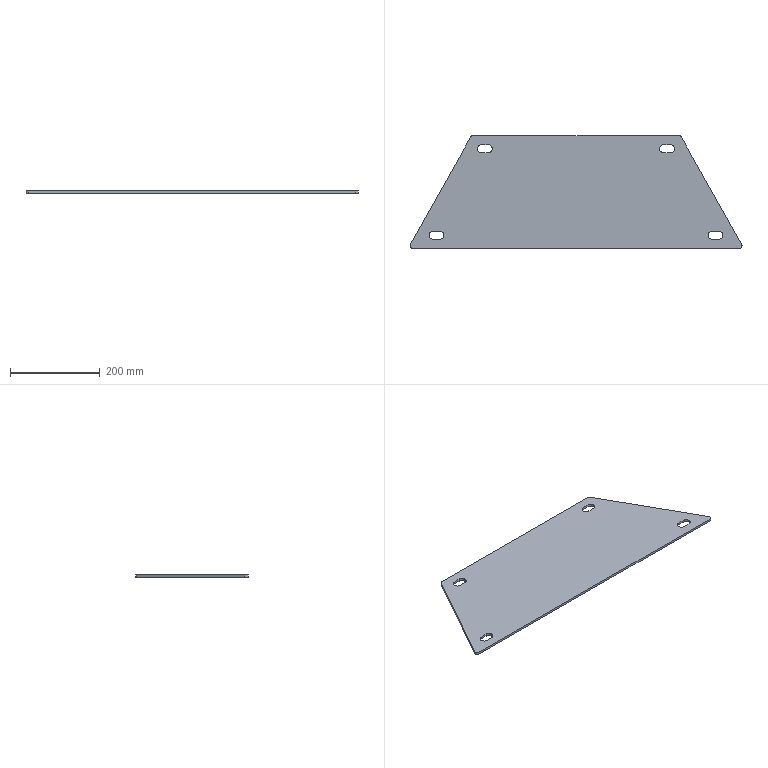Part | SolidWorks | features FlatPattern 1, SMBaseFlange 1, SheetMetal 1 | 1 solid | 31 faces | box 737.939 x 250 x 5 mm | volume 745580 mm3 | cylinder 17 | plane 14 | commonest cylinder face diameters 18 x12 10 x5
STEP:
#1=CARTESIAN_POINT('',(326.5,-96.,-5.));
#2=VERTEX_POINT('',#1);
#3=CARTESIAN_POINT('',(317.5,-87.,-5.));
#4=VERTEX_POINT('',#3);
#5=CARTESIAN_POINT('',(317.5,-96.,-5.));
#6=DIRECTION('',(0.,0.,1.));
#7=DIRECTION('',(1.,0.,0.));
#8=AXIS2_PLACEMENT_3D('',#5,#6,#7);
#9=CIRCLE('',#8,9.);
#10=EDGE_CURVE('',#2,#4,#9,.T.);
#11=ORIENTED_EDGE('',*,*,#10,.F.);
#12=CARTESIAN_POINT('',(326.5,-96.,0.));
#13=VERTEX_POINT('',#12);
#14=CARTESIAN_POINT('',(326.5,-96.,-5.));
#15=DIRECTION('',(0.,0.,1.));
#16=VECTOR('',#15,1000.);
#17=LINE('',#14,#16);
#18=EDGE_CURVE('',#2,#13,#17,.T.);
#19=ORIENTED_EDGE('',*,*,#18,.T.);
#20=CARTESIAN_POINT('',(317.5,-87.,0.));
#21=VERTEX_POINT('',#20);
#22=CARTESIAN_POINT('',(317.5,-96.,0.));
#23=DIRECTION('',(0.,0.,1.));
#24=DIRECTION('',(1.,0.,0.));
#25=AXIS2_PLACEMENT_3D('',#22,#23,#24);
#26=CIRCLE('',#25,9.);
#27=EDGE_CURVE('',#13,#21,#26,.T.);
#28=ORIENTED_EDGE('',*,*,#27,.T.);
#29=CARTESIAN_POINT('',(317.5,-87.,-5.));
#30=DIRECTION('',(0.,0.,1.));
#31=VECTOR('',#30,1000.);
#32=LINE('',#29,#31);
#33=EDGE_CURVE('',#4,#21,#32,.T.);
#34=ORIENTED_EDGE('',*,*,#33,.F.);
#35=EDGE_LOOP('',(#11,#19,#28,#34));
#36=FACE_OUTER_BOUND('',#35,.T.);
#37=CARTESIAN_POINT('',(317.5,-96.,-5.));
#38=DIRECTION('',(0.,0.,1.));
#39=DIRECTION('',(1.,0.,0.));
#40=AXIS2_PLACEMENT_3D('',#37,#38,#39);
#41=CYLINDRICAL_SURFACE('',#40,9.);
#42=ADVANCED_FACE('',(#36),#41,.F.);
#43=CARTESIAN_POINT('',(-293.5,-96.,-5.));
#44=VERTEX_POINT('',#43);
#45=CARTESIAN_POINT('',(-302.5,-87.,-5.));
#46=VERTEX_POINT('',#45);
#47=CARTESIAN_POINT('',(-302.5,-96.,-5.));
#48=DIRECTION('',(0.,0.,1.));
#49=DIRECTION('',(1.,0.,0.));
#50=AXIS2_PLACEMENT_3D('',#47,#48,#49);
#51=CIRCLE('',#50,9.);
#52=EDGE_CURVE('',#44,#46,#51,.T.);
#53=ORIENTED_EDGE('',*,*,#52,.F.);
#54=CARTESIAN_POINT('',(-293.5,-96.,0.));
#55=VERTEX_POINT('',#54);
#56=CARTESIAN_POINT('',(-293.5,-96.,-5.));
#57=DIRECTION('',(0.,0.,1.));
#58=VECTOR('',#57,1000.);
#59=LINE('',#56,#58);
#60=EDGE_CURVE('',#44,#55,#59,.T.);
#61=ORIENTED_EDGE('',*,*,#60,.T.);
#62=CARTESIAN_POINT('',(-302.5,-87.,0.));
#63=VERTEX_POINT('',#62);
#64=CARTESIAN_POINT('',(-302.5,-96.,0.));
#65=DIRECTION('',(0.,0.,1.));
#66=DIRECTION('',(1.,0.,0.));
#67=AXIS2_PLACEMENT_3D('',#64,#65,#66);
#68=CIRCLE('',#67,9.);
#69=EDGE_CURVE('',#55,#63,#68,.T.);
#70=ORIENTED_EDGE('',*,*,#69,.T.);
#71=CARTESIAN_POINT('',(-302.5,-87.,-5.));
#72=DIRECTION('',(0.,0.,1.));
#73=VECTOR('',#72,1000.);
#74=LINE('',#71,#73);
#75=EDGE_CURVE('',#46,#63,#74,.T.);
#76=ORIENTED_EDGE('',*,*,#75,.F.);
#77=EDGE_LOOP('',(#53,#61,#70,#76));
#78=FACE_OUTER_BOUND('',#77,.T.);
#79=CARTESIAN_POINT('',(-302.5,-96.,-5.));
#80=DIRECTION('',(0.,0.,1.));
#81=DIRECTION('',(1.,0.,0.));
#82=AXIS2_PLACEMENT_3D('',#79,#80,#81);
#83=CYLINDRICAL_SURFACE('',#82,9.);
#84=ADVANCED_FACE('',(#78),#83,.F.);
#85=CARTESIAN_POINT('',(219.,96.,-5.));
#86=VERTEX_POINT('',#85);
#87=CARTESIAN_POINT('',(210.,105.,-5.));
#88=VERTEX_POINT('',#87);
#89=CARTESIAN_POINT('',(210.,96.,-5.));
#90=DIRECTION('',(0.,0.,1.));
#91=DIRECTION('',(1.,0.,0.));
#92=AXIS2_PLACEMENT_3D('',#89,#90,#91);
#93=CIRCLE('',#92,9.);
#94=EDGE_CURVE('',#86,#88,#93,.T.);
#95=ORIENTED_EDGE('',*,*,#94,.F.);
#96=CARTESIAN_POINT('',(219.,96.,0.));
#97=VERTEX_POINT('',#96);
#98=CARTESIAN_POINT('',(219.,96.,-5.));
#99=DIRECTION('',(0.,0.,1.));
#100=VECTOR('',#99,1000.);
#101=LINE('',#98,#100);
#102=EDGE_CURVE('',#86,#97,#101,.T.);
#103=ORIENTED_EDGE('',*,*,#102,.T.);
#104=CARTESIAN_POINT('',(210.,105.,0.));
#105=VERTEX_POINT('',#104);
#106=CARTESIAN_POINT('',(210.,96.,0.));
#107=DIRECTION('',(0.,0.,1.));
#108=DIRECTION('',(1.,0.,0.));
#109=AXIS2_PLACEMENT_3D('',#106,#107,#108);
#110=CIRCLE('',#109,9.);
#111=EDGE_CURVE('',#97,#105,#110,.T.);
#112=ORIENTED_EDGE('',*,*,#111,.T.);
#113=CARTESIAN_POINT('',(210.,105.,-5.));
#114=DIRECTION('',(0.,0.,1.));
#115=VECTOR('',#114,1000.);
#116=LINE('',#113,#115);
#117=EDGE_CURVE('',#88,#105,#116,.T.);
#118=ORIENTED_EDGE('',*,*,#117,.F.);
#119=EDGE_LOOP('',(#95,#103,#112,#118));
#120=FACE_OUTER_BOUND('',#119,.T.);
#121=CARTESIAN_POINT('',(210.,96.,-5.));
#122=DIRECTION('',(0.,0.,1.));
#123=DIRECTION('',(1.,0.,0.));
#124=AXIS2_PLACEMENT_3D('',#121,#122,#123);
#125=CYLINDRICAL_SURFACE('',#124,9.);
#126=ADVANCED_FACE('',(#120),#125,.F.);
#127=CARTESIAN_POINT('',(-186.,96.,-5.));
#128=VERTEX_POINT('',#127);
#129=CARTESIAN_POINT('',(-195.,105.,-5.));
#130=VERTEX_POINT('',#129);
#131=CARTESIAN_POINT('',(-195.,96.,-5.));
#132=DIRECTION('',(0.,0.,1.));
#133=DIRECTION('',(1.,0.,0.));
#134=AXIS2_PLACEMENT_3D('',#131,#132,#133);
#135=CIRCLE('',#134,9.);
#136=EDGE_CURVE('',#128,#130,#135,.T.);
#137=ORIENTED_EDGE('',*,*,#136,.F.);
#138=CARTESIAN_POINT('',(-186.,96.,0.));
#139=VERTEX_POINT('',#138);
#140=CARTESIAN_POINT('',(-186.,96.,-5.));
#141=DIRECTION('',(0.,0.,1.));
#142=VECTOR('',#141,1000.);
#143=LINE('',#140,#142);
#144=EDGE_CURVE('',#128,#139,#143,.T.);
#145=ORIENTED_EDGE('',*,*,#144,.T.);
#146=CARTESIAN_POINT('',(-195.,105.,0.));
#147=VERTEX_POINT('',#146);
#148=CARTESIAN_POINT('',(-195.,96.,0.));
#149=DIRECTION('',(0.,0.,1.));
#150=DIRECTION('',(1.,0.,0.));
#151=AXIS2_PLACEMENT_3D('',#148,#149,#150);
#152=CIRCLE('',#151,9.);
#153=EDGE_CURVE('',#139,#147,#152,.T.);
#154=ORIENTED_EDGE('',*,*,#153,.T.);
#155=CARTESIAN_POINT('',(-195.,105.,-5.));
#156=DIRECTION('',(0.,0.,1.));
#157=VECTOR('',#156,1000.);
#158=LINE('',#155,#157);
#159=EDGE_CURVE('',#130,#147,#158,.T.);
#160=ORIENTED_EDGE('',*,*,#159,.F.);
#161=EDGE_LOOP('',(#137,#145,#154,#160));
#162=FACE_OUTER_BOUND('',#161,.T.);
#163=CARTESIAN_POINT('',(-195.,96.,-5.));
#164=DIRECTION('',(0.,0.,1.));
#165=DIRECTION('',(1.,0.,0.));
#166=AXIS2_PLACEMENT_3D('',#163,#164,#165);
#167=CYLINDRICAL_SURFACE('',#166,9.);
#168=ADVANCED_FACE('',(#162),#167,.F.);
#169=CARTESIAN_POINT('',(363.969,-125.,-5.));
#170=VERTEX_POINT('',#169);
#171=CARTESIAN_POINT('',(368.969,-120.,-5.));
#172=VERTEX_POINT('',#171);
#173=CARTESIAN_POINT('',(363.969,-120.,-5.));
#174=DIRECTION('',(0.,0.,1.));
#175=DIRECTION('',(-1.,0.,0.));
#176=AXIS2_PLACEMENT_3D('',#173,#174,#175);
#177=CIRCLE('',#176,5.);
#178=EDGE_CURVE('',#170,#172,#177,.T.);
#179=ORIENTED_EDGE('',*,*,#178,.T.);
#180=CARTESIAN_POINT('',(368.969,-120.,0.));
#181=VERTEX_POINT('',#180);
#182=CARTESIAN_POINT('',(368.969,-120.,-5.));
#183=DIRECTION('',(0.,0.,1.));
#184=VECTOR('',#183,1000.);
#185=LINE('',#182,#184);
#186=EDGE_CURVE('',#172,#181,#185,.T.);
#187=ORIENTED_EDGE('',*,*,#186,.T.);
#188=CARTESIAN_POINT('',(363.969,-125.,0.));
#189=VERTEX_POINT('',#188);
#190=CARTESIAN_POINT('',(363.969,-120.,0.));
#191=DIRECTION('',(0.,0.,1.));
#192=DIRECTION('',(-1.,0.,0.));
#193=AXIS2_PLACEMENT_3D('',#190,#191,#192);
#194=CIRCLE('',#193,5.);
#195=EDGE_CURVE('',#189,#181,#194,.T.);
#196=ORIENTED_EDGE('',*,*,#195,.F.);
#197=CARTESIAN_POINT('',(363.969,-125.,-5.));
#198=DIRECTION('',(0.,0.,1.));
#199=VECTOR('',#198,1000.);
#200=LINE('',#197,#199);
#201=EDGE_CURVE('',#170,#189,#200,.T.);
#202=ORIENTED_EDGE('',*,*,#201,.F.);
#203=EDGE_LOOP('',(#179,#187,#196,#202));
#204=FACE_OUTER_BOUND('',#203,.T.);
#205=CARTESIAN_POINT('',(363.969,-120.,-5.));
#206=DIRECTION('',(0.,0.,1.));
#207=DIRECTION('',(1.,0.,0.));
#208=AXIS2_PLACEMENT_3D('',#205,#206,#207);
#209=CYLINDRICAL_SURFACE('',#208,5.);
#210=ADVANCED_FACE('',(#204),#209,.T.);
#211=CARTESIAN_POINT('',(-229.569,125.,0.));
#212=VERTEX_POINT('',#211);
#213=CARTESIAN_POINT('',(-233.932,122.443,0.));
#214=VERTEX_POINT('',#213);
#215=CARTESIAN_POINT('',(-229.569,120.,0.));
#216=DIRECTION('',(0.,0.,1.));
#217=DIRECTION('',(1.,0.,0.));
#218=AXIS2_PLACEMENT_3D('',#215,#216,#217);
#219=CIRCLE('',#218,5.);
#220=EDGE_CURVE('',#212,#214,#219,.T.);
#221=ORIENTED_EDGE('',*,*,#220,.F.);
#222=CARTESIAN_POINT('',(-229.569,125.,-5.));
#223=VERTEX_POINT('',#222);
#224=CARTESIAN_POINT('',(-229.569,125.,-5.));
#225=DIRECTION('',(0.,0.,1.));
#226=VECTOR('',#225,1000.);
#227=LINE('',#224,#226);
#228=EDGE_CURVE('',#223,#212,#227,.T.);
#229=ORIENTED_EDGE('',*,*,#228,.F.);
#230=CARTESIAN_POINT('',(-233.932,122.443,-5.));
#231=VERTEX_POINT('',#230);
#232=CARTESIAN_POINT('',(-229.569,120.,-5.));
#233=DIRECTION('',(0.,0.,1.));
#234=DIRECTION('',(1.,0.,0.));
#235=AXIS2_PLACEMENT_3D('',#232,#233,#234);
#236=CIRCLE('',#235,5.);
#237=EDGE_CURVE('',#223,#231,#236,.T.);
#238=ORIENTED_EDGE('',*,*,#237,.T.);
#239=CARTESIAN_POINT('',(-233.932,122.443,-5.));
#240=DIRECTION('',(0.,0.,1.));
#241=VECTOR('',#240,1000.);
#242=LINE('',#239,#241);
#243=EDGE_CURVE('',#231,#214,#242,.T.);
#244=ORIENTED_EDGE('',*,*,#243,.T.);
#245=EDGE_LOOP('',(#221,#229,#238,#244));
#246=FACE_OUTER_BOUND('',#245,.T.);
#247=CARTESIAN_POINT('',(-229.569,120.,-5.));
#248=DIRECTION('',(0.,0.,1.));
#249=DIRECTION('',(1.,0.,0.));
#250=AXIS2_PLACEMENT_3D('',#247,#248,#249);
#251=CYLINDRICAL_SURFACE('',#250,5.);
#252=ADVANCED_FACE('',(#246),#251,.T.);
#253=CARTESIAN_POINT('',(229.569,125.,0.));
#254=VERTEX_POINT('',#253);
#255=CARTESIAN_POINT('',(-229.569,125.,0.));
#256=DIRECTION('',(-1.,0.,0.));
#257=VECTOR('',#256,1000.);
#258=LINE('',#255,#257);
#259=EDGE_CURVE('',#254,#212,#258,.T.);
#260=ORIENTED_EDGE('',*,*,#259,.F.);
#261=CARTESIAN_POINT('',(229.569,125.,-5.));
#262=VERTEX_POINT('',#261);
#263=CARTESIAN_POINT('',(229.569,125.,-5.));
#264=DIRECTION('',(0.,0.,1.));
#265=VECTOR('',#264,1000.);
#266=LINE('',#263,#265);
#267=EDGE_CURVE('',#262,#254,#266,.T.);
#268=ORIENTED_EDGE('',*,*,#267,.F.);
#269=CARTESIAN_POINT('',(-229.569,125.,-5.));
#270=DIRECTION('',(-1.,0.,0.));
#271=VECTOR('',#270,1000.);
#272=LINE('',#269,#271);
#273=EDGE_CURVE('',#262,#223,#272,.T.);
#274=ORIENTED_EDGE('',*,*,#273,.T.);
#275=ORIENTED_EDGE('',*,*,#228,.T.);
#276=EDGE_LOOP('',(#260,#268,#274,#275));
#277=FACE_OUTER_BOUND('',#276,.T.);
#278=CARTESIAN_POINT('',(-229.569,125.,-5.));
#279=DIRECTION('',(0.,1.,0.));
#280=DIRECTION('',(0.,0.,1.));
#281=AXIS2_PLACEMENT_3D('',#278,#279,#280);
#282=PLANE('',#281);
#283=ADVANCED_FACE('',(#277),#282,.T.);
#284=CARTESIAN_POINT('',(233.932,122.443,0.));
#285=VERTEX_POINT('',#284);
#286=CARTESIAN_POINT('',(229.569,120.,0.));
#287=DIRECTION('',(0.,0.,1.));
#288=DIRECTION('',(-1.,0.,0.));
#289=AXIS2_PLACEMENT_3D('',#286,#287,#288);
#290=CIRCLE('',#289,5.);
#291=EDGE_CURVE('',#285,#254,#290,.T.);
#292=ORIENTED_EDGE('',*,*,#291,.F.);
#293=CARTESIAN_POINT('',(233.932,122.443,-5.));
#294=VERTEX_POINT('',#293);
#295=CARTESIAN_POINT('',(233.932,122.443,-5.));
#296=DIRECTION('',(0.,0.,1.));
#297=VECTOR('',#296,1000.);
#298=LINE('',#295,#297);
#299=EDGE_CURVE('',#294,#285,#298,.T.);
#300=ORIENTED_EDGE('',*,*,#299,.F.);
#301=CARTESIAN_POINT('',(229.569,120.,-5.));
#302=DIRECTION('',(0.,0.,1.));
#303=DIRECTION('',(-1.,0.,0.));
#304=AXIS2_PLACEMENT_3D('',#301,#302,#303);
#305=CIRCLE('',#304,5.);
#306=EDGE_CURVE('',#294,#262,#305,.T.);
#307=ORIENTED_EDGE('',*,*,#306,.T.);
#308=ORIENTED_EDGE('',*,*,#267,.T.);
#309=EDGE_LOOP('',(#292,#300,#307,#308));
#310=FACE_OUTER_BOUND('',#309,.T.);
#311=CARTESIAN_POINT('',(229.569,120.,-5.));
#312=DIRECTION('',(0.,0.,1.));
#313=DIRECTION('',(1.,0.,0.));
#314=AXIS2_PLACEMENT_3D('',#311,#312,#313);
#315=CYLINDRICAL_SURFACE('',#314,5.);
#316=ADVANCED_FACE('',(#310),#315,.T.);
#317=CARTESIAN_POINT('',(368.332,-117.557,0.));
#318=VERTEX_POINT('',#317);
#319=CARTESIAN_POINT('',(233.932,122.443,0.));
#320=DIRECTION('',(-0.4886,0.8725,0.));
#321=VECTOR('',#320,1000.);
#322=LINE('',#319,#321);
#323=EDGE_CURVE('',#318,#285,#322,.T.);
#324=ORIENTED_EDGE('',*,*,#323,.F.);
#325=CARTESIAN_POINT('',(368.332,-117.557,-5.));
#326=VERTEX_POINT('',#325);
#327=CARTESIAN_POINT('',(368.332,-117.557,-5.));
#328=DIRECTION('',(0.,0.,1.));
#329=VECTOR('',#328,1000.);
#330=LINE('',#327,#329);
#331=EDGE_CURVE('',#326,#318,#330,.T.);
#332=ORIENTED_EDGE('',*,*,#331,.F.);
#333=CARTESIAN_POINT('',(233.932,122.443,-5.));
#334=DIRECTION('',(-0.4886,0.8725,0.));
#335=VECTOR('',#334,1000.);
#336=LINE('',#333,#335);
#337=EDGE_CURVE('',#326,#294,#336,.T.);
#338=ORIENTED_EDGE('',*,*,#337,.T.);
#339=ORIENTED_EDGE('',*,*,#299,.T.);
#340=EDGE_LOOP('',(#324,#332,#338,#339));
#341=FACE_OUTER_BOUND('',#340,.T.);
#342=CARTESIAN_POINT('',(233.932,122.443,-5.));
#343=DIRECTION('',(0.8725,0.4886,0.));
#344=DIRECTION('',(-0.4886,0.8725,0.));
#345=AXIS2_PLACEMENT_3D('',#342,#343,#344);
#346=PLANE('',#345);
#347=ADVANCED_FACE('',(#341),#346,.T.);
#348=ORIENTED_EDGE('',*,*,#186,.F.);
#349=CARTESIAN_POINT('',(363.969,-120.,-5.));
#350=DIRECTION('',(0.,0.,1.));
#351=DIRECTION('',(-1.,0.,0.));
#352=AXIS2_PLACEMENT_3D('',#349,#350,#351);
#353=CIRCLE('',#352,5.);
#354=EDGE_CURVE('',#172,#326,#353,.T.);
#355=ORIENTED_EDGE('',*,*,#354,.T.);
#356=ORIENTED_EDGE('',*,*,#331,.T.);
#357=CARTESIAN_POINT('',(363.969,-120.,0.));
#358=DIRECTION('',(0.,0.,1.));
#359=DIRECTION('',(-1.,0.,0.));
#360=AXIS2_PLACEMENT_3D('',#357,#358,#359);
#361=CIRCLE('',#360,5.);
#362=EDGE_CURVE('',#181,#318,#361,.T.);
#363=ORIENTED_EDGE('',*,*,#362,.F.);
#364=EDGE_LOOP('',(#348,#355,#356,#363));
#365=FACE_OUTER_BOUND('',#364,.T.);
#366=CARTESIAN_POINT('',(363.969,-120.,-5.));
#367=DIRECTION('',(0.,0.,1.));
#368=DIRECTION('',(1.,0.,0.));
#369=AXIS2_PLACEMENT_3D('',#366,#367,#368);
#370=CYLINDRICAL_SURFACE('',#369,5.);
#371=ADVANCED_FACE('',(#365),#370,.T.);
#372=CARTESIAN_POINT('',(-363.969,-125.,0.));
#373=VERTEX_POINT('',#372);
#374=CARTESIAN_POINT('',(363.969,-125.,0.));
#375=DIRECTION('',(1.,0.,0.));
#376=VECTOR('',#375,1000.);
#377=LINE('',#374,#376);
#378=EDGE_CURVE('',#373,#189,#377,.T.);
#379=ORIENTED_EDGE('',*,*,#378,.F.);
#380=CARTESIAN_POINT('',(-363.969,-125.,-5.));
#381=VERTEX_POINT('',#380);
#382=CARTESIAN_POINT('',(-363.969,-125.,-5.));
#383=DIRECTION('',(0.,0.,1.));
#384=VECTOR('',#383,1000.);
#385=LINE('',#382,#384);
#386=EDGE_CURVE('',#381,#373,#385,.T.);
#387=ORIENTED_EDGE('',*,*,#386,.F.);
#388=CARTESIAN_POINT('',(363.969,-125.,-5.));
#389=DIRECTION('',(1.,0.,0.));
#390=VECTOR('',#389,1000.);
#391=LINE('',#388,#390);
#392=EDGE_CURVE('',#381,#170,#391,.T.);
#393=ORIENTED_EDGE('',*,*,#392,.T.);
#394=ORIENTED_EDGE('',*,*,#201,.T.);
#395=EDGE_LOOP('',(#379,#387,#393,#394));
#396=FACE_OUTER_BOUND('',#395,.T.);
#397=CARTESIAN_POINT('',(363.969,-125.,-5.));
#398=DIRECTION('',(0.,-1.,0.));
#399=DIRECTION('',(1.,0.,0.));
#400=AXIS2_PLACEMENT_3D('',#397,#398,#399);
#401=PLANE('',#400);
#402=ADVANCED_FACE('',(#396),#401,.T.);
#403=CARTESIAN_POINT('',(-368.332,-117.557,0.));
#404=VERTEX_POINT('',#403);
#405=CARTESIAN_POINT('',(-363.969,-120.,0.));
#406=DIRECTION('',(0.,0.,1.));
#407=DIRECTION('',(-1.,0.,0.));
#408=AXIS2_PLACEMENT_3D('',#405,#406,#407);
#409=CIRCLE('',#408,5.);
#410=EDGE_CURVE('',#404,#373,#409,.T.);
#411=ORIENTED_EDGE('',*,*,#410,.F.);
#412=CARTESIAN_POINT('',(-368.332,-117.557,-5.));
#413=VERTEX_POINT('',#412);
#414=CARTESIAN_POINT('',(-368.332,-117.557,-5.));
#415=DIRECTION('',(0.,0.,1.));
#416=VECTOR('',#415,1000.);
#417=LINE('',#414,#416);
#418=EDGE_CURVE('',#413,#404,#417,.T.);
#419=ORIENTED_EDGE('',*,*,#418,.F.);
#420=CARTESIAN_POINT('',(-363.969,-120.,-5.));
#421=DIRECTION('',(0.,0.,1.));
#422=DIRECTION('',(-1.,0.,0.));
#423=AXIS2_PLACEMENT_3D('',#420,#421,#422);
#424=CIRCLE('',#423,5.);
#425=EDGE_CURVE('',#413,#381,#424,.T.);
#426=ORIENTED_EDGE('',*,*,#425,.T.);
#427=ORIENTED_EDGE('',*,*,#386,.T.);
#428=EDGE_LOOP('',(#411,#419,#426,#427));
#429=FACE_OUTER_BOUND('',#428,.T.);
#430=CARTESIAN_POINT('',(-363.969,-120.,-5.));
#431=DIRECTION('',(0.,0.,1.));
#432=DIRECTION('',(1.,0.,0.));
#433=AXIS2_PLACEMENT_3D('',#430,#431,#432);
#434=CYLINDRICAL_SURFACE('',#433,5.);
#435=ADVANCED_FACE('',(#429),#434,.T.);
#436=CARTESIAN_POINT('',(-368.332,-117.557,0.));
#437=DIRECTION('',(-0.4886,-0.8725,0.));
#438=VECTOR('',#437,1000.);
#439=LINE('',#436,#438);
#440=EDGE_CURVE('',#214,#404,#439,.T.);
#441=ORIENTED_EDGE('',*,*,#440,.F.);
#442=ORIENTED_EDGE('',*,*,#243,.F.);
#443=CARTESIAN_POINT('',(-368.332,-117.557,-5.));
#444=DIRECTION('',(-0.4886,-0.8725,0.));
#445=VECTOR('',#444,1000.);
#446=LINE('',#443,#445);
#447=EDGE_CURVE('',#231,#413,#446,.T.);
#448=ORIENTED_EDGE('',*,*,#447,.T.);
#449=ORIENTED_EDGE('',*,*,#418,.T.);
#450=EDGE_LOOP('',(#441,#442,#448,#449));
#451=FACE_OUTER_BOUND('',#450,.T.);
#452=CARTESIAN_POINT('',(-368.332,-117.557,-5.));
#453=DIRECTION('',(-0.8725,0.4886,0.));
#454=DIRECTION('',(-0.4886,-0.8725,0.));
#455=AXIS2_PLACEMENT_3D('',#452,#453,#454);
#456=PLANE('',#455);
#457=ADVANCED_FACE('',(#451),#456,.T.);
#458=CARTESIAN_POINT('',(302.5,-105.,-5.));
#459=VERTEX_POINT('',#458);
#460=CARTESIAN_POINT('',(317.5,-105.,-5.));
#461=VERTEX_POINT('',#460);
#462=CARTESIAN_POINT('',(317.5,-105.,-5.));
#463=DIRECTION('',(1.,0.,0.));
#464=VECTOR('',#463,1000.);
#465=LINE('',#462,#464);
#466=EDGE_CURVE('',#459,#461,#465,.T.);
#467=ORIENTED_EDGE('',*,*,#466,.T.);
#468=CARTESIAN_POINT('',(317.5,-96.,-5.));
#469=DIRECTION('',(0.,0.,1.));
#470=DIRECTION('',(1.,0.,0.));
#471=AXIS2_PLACEMENT_3D('',#468,#469,#470);
#472=CIRCLE('',#471,9.);
#473=EDGE_CURVE('',#461,#2,#472,.T.);
#474=ORIENTED_EDGE('',*,*,#473,.T.);
#475=ORIENTED_EDGE('',*,*,#10,.T.);
#476=CARTESIAN_POINT('',(302.5,-87.,-5.));
#477=VERTEX_POINT('',#476);
#478=CARTESIAN_POINT('',(317.5,-87.,-5.));
#479=DIRECTION('',(-1.,0.,0.));
#480=VECTOR('',#479,1000.);
#481=LINE('',#478,#480);
#482=EDGE_CURVE('',#4,#477,#481,.T.);
#483=ORIENTED_EDGE('',*,*,#482,.T.);
#484=CARTESIAN_POINT('',(302.5,-96.,-5.));
#485=DIRECTION('',(0.,0.,1.));
#486=DIRECTION('',(1.,0.,0.));
#487=AXIS2_PLACEMENT_3D('',#484,#485,#486);
#488=CIRCLE('',#487,9.);
#489=EDGE_CURVE('',#477,#459,#488,.T.);
#490=ORIENTED_EDGE('',*,*,#489,.T.);
#491=EDGE_LOOP('',(#467,#474,#475,#483,#490));
#492=FACE_BOUND('',#491,.T.);
#493=CARTESIAN_POINT('',(-317.5,-87.,-5.));
#494=VERTEX_POINT('',#493);
#495=CARTESIAN_POINT('',(-317.5,-87.,-5.));
#496=DIRECTION('',(-1.,0.,0.));
#497=VECTOR('',#496,1000.);
#498=LINE('',#495,#497);
#499=EDGE_CURVE('',#46,#494,#498,.T.);
#500=ORIENTED_EDGE('',*,*,#499,.T.);
#501=CARTESIAN_POINT('',(-317.5,-105.,-5.));
#502=VERTEX_POINT('',#501);
#503=CARTESIAN_POINT('',(-317.5,-96.,-5.));
#504=DIRECTION('',(0.,0.,1.));
#505=DIRECTION('',(1.,0.,0.));
#506=AXIS2_PLACEMENT_3D('',#503,#504,#505);
#507=CIRCLE('',#506,9.);
#508=EDGE_CURVE('',#494,#502,#507,.T.);
#509=ORIENTED_EDGE('',*,*,#508,.T.);
#510=CARTESIAN_POINT('',(-302.5,-105.,-5.));
#511=VERTEX_POINT('',#510);
#512=CARTESIAN_POINT('',(-317.5,-105.,-5.));
#513=DIRECTION('',(1.,0.,0.));
#514=VECTOR('',#513,1000.);
#515=LINE('',#512,#514);
#516=EDGE_CURVE('',#502,#511,#515,.T.);
#517=ORIENTED_EDGE('',*,*,#516,.T.);
#518=CARTESIAN_POINT('',(-302.5,-96.,-5.));
#519=DIRECTION('',(0.,0.,1.));
#520=DIRECTION('',(1.,0.,0.));
#521=AXIS2_PLACEMENT_3D('',#518,#519,#520);
#522=CIRCLE('',#521,9.);
#523=EDGE_CURVE('',#511,#44,#522,.T.);
#524=ORIENTED_EDGE('',*,*,#523,.T.);
#525=ORIENTED_EDGE('',*,*,#52,.T.);
#526=EDGE_LOOP('',(#500,#509,#517,#524,#525));
#527=FACE_BOUND('',#526,.T.);
#528=CARTESIAN_POINT('',(195.,87.,-5.));
#529=VERTEX_POINT('',#528);
#530=CARTESIAN_POINT('',(210.,87.,-5.));
#531=VERTEX_POINT('',#530);
#532=CARTESIAN_POINT('',(210.,87.,-5.));
#533=DIRECTION('',(1.,0.,0.));
#534=VECTOR('',#533,1000.);
#535=LINE('',#532,#534);
#536=EDGE_CURVE('',#529,#531,#535,.T.);
#537=ORIENTED_EDGE('',*,*,#536,.T.);
#538=CARTESIAN_POINT('',(210.,96.,-5.));
#539=DIRECTION('',(0.,0.,1.));
#540=DIRECTION('',(1.,0.,0.));
#541=AXIS2_PLACEMENT_3D('',#538,#539,#540);
#542=CIRCLE('',#541,9.);
#543=EDGE_CURVE('',#531,#86,#542,.T.);
#544=ORIENTED_EDGE('',*,*,#543,.T.);
#545=ORIENTED_EDGE('',*,*,#94,.T.);
#546=CARTESIAN_POINT('',(195.,105.,-5.));
#547=VERTEX_POINT('',#546);
#548=CARTESIAN_POINT('',(210.,105.,-5.));
#549=DIRECTION('',(-1.,0.,0.));
#550=VECTOR('',#549,1000.);
#551=LINE('',#548,#550);
#552=EDGE_CURVE('',#88,#547,#551,.T.);
#553=ORIENTED_EDGE('',*,*,#552,.T.);
#554=CARTESIAN_POINT('',(195.,96.,-5.));
#555=DIRECTION('',(0.,0.,1.));
#556=DIRECTION('',(1.,0.,0.));
#557=AXIS2_PLACEMENT_3D('',#554,#555,#556);
#558=CIRCLE('',#557,9.);
#559=EDGE_CURVE('',#547,#529,#558,.T.);
#560=ORIENTED_EDGE('',*,*,#559,.T.);
#561=EDGE_LOOP('',(#537,#544,#545,#553,#560));
#562=FACE_BOUND('',#561,.T.);
#563=CARTESIAN_POINT('',(-210.,105.,-5.));
#564=VERTEX_POINT('',#563);
#565=CARTESIAN_POINT('',(-210.,105.,-5.));
#566=DIRECTION('',(-1.,0.,0.));
#567=VECTOR('',#566,1000.);
#568=LINE('',#565,#567);
#569=EDGE_CURVE('',#130,#564,#568,.T.);
#570=ORIENTED_EDGE('',*,*,#569,.T.);
#571=CARTESIAN_POINT('',(-210.,87.,-5.));
#572=VERTEX_POINT('',#571);
#573=CARTESIAN_POINT('',(-210.,96.,-5.));
#574=DIRECTION('',(0.,0.,1.));
#575=DIRECTION('',(1.,0.,0.));
#576=AXIS2_PLACEMENT_3D('',#573,#574,#575);
#577=CIRCLE('',#576,9.);
#578=EDGE_CURVE('',#564,#572,#577,.T.);
#579=ORIENTED_EDGE('',*,*,#578,.T.);
#580=CARTESIAN_POINT('',(-195.,87.,-5.));
#581=VERTEX_POINT('',#580);
#582=CARTESIAN_POINT('',(-210.,87.,-5.));
#583=DIRECTION('',(1.,0.,0.));
#584=VECTOR('',#583,1000.);
#585=LINE('',#582,#584);
#586=EDGE_CURVE('',#572,#581,#585,.T.);
#587=ORIENTED_EDGE('',*,*,#586,.T.);
#588=CARTESIAN_POINT('',(-195.,96.,-5.));
#589=DIRECTION('',(0.,0.,1.));
#590=DIRECTION('',(1.,0.,0.));
#591=AXIS2_PLACEMENT_3D('',#588,#589,#590);
#592=CIRCLE('',#591,9.);
#593=EDGE_CURVE('',#581,#128,#592,.T.);
#594=ORIENTED_EDGE('',*,*,#593,.T.);
#595=ORIENTED_EDGE('',*,*,#136,.T.);
#596=EDGE_LOOP('',(#570,#579,#587,#594,#595));
#597=FACE_BOUND('',#596,.T.);
#598=ORIENTED_EDGE('',*,*,#237,.F.);
#599=ORIENTED_EDGE('',*,*,#273,.F.);
#600=ORIENTED_EDGE('',*,*,#306,.F.);
#601=ORIENTED_EDGE('',*,*,#337,.F.);
#602=ORIENTED_EDGE('',*,*,#354,.F.);
#603=ORIENTED_EDGE('',*,*,#178,.F.);
#604=ORIENTED_EDGE('',*,*,#392,.F.);
#605=ORIENTED_EDGE('',*,*,#425,.F.);
#606=ORIENTED_EDGE('',*,*,#447,.F.);
#607=EDGE_LOOP('',(#598,#599,#600,#601,#602,#603,#604,#605,#606));
#608=FACE_OUTER_BOUND('',#607,.T.);
#609=CARTESIAN_POINT('',(-229.569,120.,-5.));
#610=DIRECTION('',(0.,0.,1.));
#611=DIRECTION('',(1.,0.,0.));
#612=AXIS2_PLACEMENT_3D('',#609,#610,#611);
#613=PLANE('',#612);
#614=ADVANCED_FACE('',(#492,#527,#562,#597,#608),#613,.F.);
#615=CARTESIAN_POINT('',(317.5,-105.,0.));
#616=VERTEX_POINT('',#615);
#617=CARTESIAN_POINT('',(317.5,-96.,0.));
#618=DIRECTION('',(0.,0.,1.));
#619=DIRECTION('',(1.,0.,0.));
#620=AXIS2_PLACEMENT_3D('',#617,#618,#619);
#621=CIRCLE('',#620,9.);
#622=EDGE_CURVE('',#616,#13,#621,.T.);
#623=ORIENTED_EDGE('',*,*,#622,.F.);
#624=CARTESIAN_POINT('',(302.5,-105.,0.));
#625=VERTEX_POINT('',#624);
#626=CARTESIAN_POINT('',(317.5,-105.,0.));
#627=DIRECTION('',(1.,0.,0.));
#628=VECTOR('',#627,1000.);
#629=LINE('',#626,#628);
#630=EDGE_CURVE('',#625,#616,#629,.T.);
#631=ORIENTED_EDGE('',*,*,#630,.F.);
#632=CARTESIAN_POINT('',(302.5,-87.,0.));
#633=VERTEX_POINT('',#632);
#634=CARTESIAN_POINT('',(302.5,-96.,0.));
#635=DIRECTION('',(0.,0.,1.));
#636=DIRECTION('',(1.,0.,0.));
#637=AXIS2_PLACEMENT_3D('',#634,#635,#636);
#638=CIRCLE('',#637,9.);
#639=EDGE_CURVE('',#633,#625,#638,.T.);
#640=ORIENTED_EDGE('',*,*,#639,.F.);
#641=CARTESIAN_POINT('',(317.5,-87.,0.));
#642=DIRECTION('',(-1.,0.,0.));
#643=VECTOR('',#642,1000.);
#644=LINE('',#641,#643);
#645=EDGE_CURVE('',#21,#633,#644,.T.);
#646=ORIENTED_EDGE('',*,*,#645,.F.);
#647=ORIENTED_EDGE('',*,*,#27,.F.);
#648=EDGE_LOOP('',(#623,#631,#640,#646,#647));
#649=FACE_BOUND('',#648,.T.);
#650=CARTESIAN_POINT('',(-317.5,-87.,0.));
#651=VERTEX_POINT('',#650);
#652=CARTESIAN_POINT('',(-317.5,-105.,0.));
#653=VERTEX_POINT('',#652);
#654=CARTESIAN_POINT('',(-317.5,-96.,0.));
#655=DIRECTION('',(0.,0.,1.));
#656=DIRECTION('',(1.,0.,0.));
#657=AXIS2_PLACEMENT_3D('',#654,#655,#656);
#658=CIRCLE('',#657,9.);
#659=EDGE_CURVE('',#651,#653,#658,.T.);
#660=ORIENTED_EDGE('',*,*,#659,.F.);
#661=CARTESIAN_POINT('',(-317.5,-87.,0.));
#662=DIRECTION('',(-1.,0.,0.));
#663=VECTOR('',#662,1000.);
#664=LINE('',#661,#663);
#665=EDGE_CURVE('',#63,#651,#664,.T.);
#666=ORIENTED_EDGE('',*,*,#665,.F.);
#667=ORIENTED_EDGE('',*,*,#69,.F.);
#668=CARTESIAN_POINT('',(-302.5,-105.,0.));
#669=VERTEX_POINT('',#668);
#670=CARTESIAN_POINT('',(-302.5,-96.,0.));
#671=DIRECTION('',(0.,0.,1.));
#672=DIRECTION('',(1.,0.,0.));
#673=AXIS2_PLACEMENT_3D('',#670,#671,#672);
#674=CIRCLE('',#673,9.);
#675=EDGE_CURVE('',#669,#55,#674,.T.);
#676=ORIENTED_EDGE('',*,*,#675,.F.);
#677=CARTESIAN_POINT('',(-317.5,-105.,0.));
#678=DIRECTION('',(1.,0.,0.));
#679=VECTOR('',#678,1000.);
#680=LINE('',#677,#679);
#681=EDGE_CURVE('',#653,#669,#680,.T.);
#682=ORIENTED_EDGE('',*,*,#681,.F.);
#683=EDGE_LOOP('',(#660,#666,#667,#676,#682));
#684=FACE_BOUND('',#683,.T.);
#685=CARTESIAN_POINT('',(210.,87.,0.));
#686=VERTEX_POINT('',#685);
#687=CARTESIAN_POINT('',(210.,96.,0.));
#688=DIRECTION('',(0.,0.,1.));
#689=DIRECTION('',(1.,0.,0.));
#690=AXIS2_PLACEMENT_3D('',#687,#688,#689);
#691=CIRCLE('',#690,9.);
#692=EDGE_CURVE('',#686,#97,#691,.T.);
#693=ORIENTED_EDGE('',*,*,#692,.F.);
#694=CARTESIAN_POINT('',(195.,87.,0.));
#695=VERTEX_POINT('',#694);
#696=CARTESIAN_POINT('',(210.,87.,0.));
#697=DIRECTION('',(1.,0.,0.));
#698=VECTOR('',#697,1000.);
#699=LINE('',#696,#698);
#700=EDGE_CURVE('',#695,#686,#699,.T.);
#701=ORIENTED_EDGE('',*,*,#700,.F.);
#702=CARTESIAN_POINT('',(195.,105.,0.));
#703=VERTEX_POINT('',#702);
#704=CARTESIAN_POINT('',(195.,96.,0.));
#705=DIRECTION('',(0.,0.,1.));
#706=DIRECTION('',(1.,0.,0.));
#707=AXIS2_PLACEMENT_3D('',#704,#705,#706);
#708=CIRCLE('',#707,9.);
#709=EDGE_CURVE('',#703,#695,#708,.T.);
#710=ORIENTED_EDGE('',*,*,#709,.F.);
#711=CARTESIAN_POINT('',(210.,105.,0.));
#712=DIRECTION('',(-1.,0.,0.));
#713=VECTOR('',#712,1000.);
#714=LINE('',#711,#713);
#715=EDGE_CURVE('',#105,#703,#714,.T.);
#716=ORIENTED_EDGE('',*,*,#715,.F.);
#717=ORIENTED_EDGE('',*,*,#111,.F.);
#718=EDGE_LOOP('',(#693,#701,#710,#716,#717));
#719=FACE_BOUND('',#718,.T.);
#720=CARTESIAN_POINT('',(-210.,105.,0.));
#721=VERTEX_POINT('',#720);
#722=CARTESIAN_POINT('',(-210.,87.,0.));
#723=VERTEX_POINT('',#722);
#724=CARTESIAN_POINT('',(-210.,96.,0.));
#725=DIRECTION('',(0.,0.,1.));
#726=DIRECTION('',(1.,0.,0.));
#727=AXIS2_PLACEMENT_3D('',#724,#725,#726);
#728=CIRCLE('',#727,9.);
#729=EDGE_CURVE('',#721,#723,#728,.T.);
#730=ORIENTED_EDGE('',*,*,#729,.F.);
#731=CARTESIAN_POINT('',(-210.,105.,0.));
#732=DIRECTION('',(-1.,0.,0.));
#733=VECTOR('',#732,1000.);
#734=LINE('',#731,#733);
#735=EDGE_CURVE('',#147,#721,#734,.T.);
#736=ORIENTED_EDGE('',*,*,#735,.F.);
#737=ORIENTED_EDGE('',*,*,#153,.F.);
#738=CARTESIAN_POINT('',(-195.,87.,0.));
#739=VERTEX_POINT('',#738);
#740=CARTESIAN_POINT('',(-195.,96.,0.));
#741=DIRECTION('',(0.,0.,1.));
#742=DIRECTION('',(1.,0.,0.));
#743=AXIS2_PLACEMENT_3D('',#740,#741,#742);
#744=CIRCLE('',#743,9.);
#745=EDGE_CURVE('',#739,#139,#744,.T.);
#746=ORIENTED_EDGE('',*,*,#745,.F.);
#747=CARTESIAN_POINT('',(-210.,87.,0.));
#748=DIRECTION('',(1.,0.,0.));
#749=VECTOR('',#748,1000.);
#750=LINE('',#747,#749);
#751=EDGE_CURVE('',#723,#739,#750,.T.);
#752=ORIENTED_EDGE('',*,*,#751,.F.);
#753=EDGE_LOOP('',(#730,#736,#737,#746,#752));
#754=FACE_BOUND('',#753,.T.);
#755=ORIENTED_EDGE('',*,*,#220,.T.);
#756=ORIENTED_EDGE('',*,*,#440,.T.);
#757=ORIENTED_EDGE('',*,*,#410,.T.);
#758=ORIENTED_EDGE('',*,*,#378,.T.);
#759=ORIENTED_EDGE('',*,*,#195,.T.);
#760=ORIENTED_EDGE('',*,*,#362,.T.);
#761=ORIENTED_EDGE('',*,*,#323,.T.);
#762=ORIENTED_EDGE('',*,*,#291,.T.);
#763=ORIENTED_EDGE('',*,*,#259,.T.);
#764=EDGE_LOOP('',(#755,#756,#757,#758,#759,#760,#761,#762,#763));
#765=FACE_OUTER_BOUND('',#764,.T.);
#766=CARTESIAN_POINT('',(-229.569,120.,0.));
#767=DIRECTION('',(0.,0.,1.));
#768=DIRECTION('',(1.,0.,0.));
#769=AXIS2_PLACEMENT_3D('',#766,#767,#768);
#770=PLANE('',#769);
#771=ADVANCED_FACE('',(#649,#684,#719,#754,#765),#770,.T.);
#772=ORIENTED_EDGE('',*,*,#729,.T.);
#773=CARTESIAN_POINT('',(-210.,87.,-5.));
#774=DIRECTION('',(0.,0.,1.));
#775=VECTOR('',#774,1000.);
#776=LINE('',#773,#775);
#777=EDGE_CURVE('',#572,#723,#776,.T.);
#778=ORIENTED_EDGE('',*,*,#777,.F.);
#779=ORIENTED_EDGE('',*,*,#578,.F.);
#780=CARTESIAN_POINT('',(-210.,105.,-5.));
#781=DIRECTION('',(0.,0.,1.));
#782=VECTOR('',#781,1000.);
#783=LINE('',#780,#782);
#784=EDGE_CURVE('',#564,#721,#783,.T.);
#785=ORIENTED_EDGE('',*,*,#784,.T.);
#786=EDGE_LOOP('',(#772,#778,#779,#785));
#787=FACE_OUTER_BOUND('',#786,.T.);
#788=CARTESIAN_POINT('',(-210.,96.,-5.));
#789=DIRECTION('',(0.,0.,1.));
#790=DIRECTION('',(1.,0.,0.));
#791=AXIS2_PLACEMENT_3D('',#788,#789,#790);
#792=CYLINDRICAL_SURFACE('',#791,9.);
#793=ADVANCED_FACE('',(#787),#792,.F.);
#794=ORIENTED_EDGE('',*,*,#735,.T.);
#795=ORIENTED_EDGE('',*,*,#784,.F.);
#796=ORIENTED_EDGE('',*,*,#569,.F.);
#797=ORIENTED_EDGE('',*,*,#159,.T.);
#798=EDGE_LOOP('',(#794,#795,#796,#797));
#799=FACE_OUTER_BOUND('',#798,.T.);
#800=CARTESIAN_POINT('',(-210.,105.,-5.));
#801=DIRECTION('',(0.,1.,0.));
#802=DIRECTION('',(0.,0.,1.));
#803=AXIS2_PLACEMENT_3D('',#800,#801,#802);
#804=PLANE('',#803);
#805=ADVANCED_FACE('',(#799),#804,.F.);
#806=ORIENTED_EDGE('',*,*,#144,.F.);
#807=ORIENTED_EDGE('',*,*,#593,.F.);
#808=CARTESIAN_POINT('',(-195.,87.,-5.));
#809=DIRECTION('',(0.,0.,1.));
#810=VECTOR('',#809,1000.);
#811=LINE('',#808,#810);
#812=EDGE_CURVE('',#581,#739,#811,.T.);
#813=ORIENTED_EDGE('',*,*,#812,.T.);
#814=ORIENTED_EDGE('',*,*,#745,.T.);
#815=EDGE_LOOP('',(#806,#807,#813,#814));
#816=FACE_OUTER_BOUND('',#815,.T.);
#817=CARTESIAN_POINT('',(-195.,96.,-5.));
#818=DIRECTION('',(0.,0.,1.));
#819=DIRECTION('',(1.,0.,0.));
#820=AXIS2_PLACEMENT_3D('',#817,#818,#819);
#821=CYLINDRICAL_SURFACE('',#820,9.);
#822=ADVANCED_FACE('',(#816),#821,.F.);
#823=ORIENTED_EDGE('',*,*,#751,.T.);
#824=ORIENTED_EDGE('',*,*,#812,.F.);
#825=ORIENTED_EDGE('',*,*,#586,.F.);
#826=ORIENTED_EDGE('',*,*,#777,.T.);
#827=EDGE_LOOP('',(#823,#824,#825,#826));
#828=FACE_OUTER_BOUND('',#827,.T.);
#829=CARTESIAN_POINT('',(-210.,87.,-5.));
#830=DIRECTION('',(0.,-1.,0.));
#831=DIRECTION('',(0.,0.,-1.));
#832=AXIS2_PLACEMENT_3D('',#829,#830,#831);
#833=PLANE('',#832);
#834=ADVANCED_FACE('',(#828),#833,.F.);
#835=ORIENTED_EDGE('',*,*,#102,.F.);
#836=ORIENTED_EDGE('',*,*,#543,.F.);
#837=CARTESIAN_POINT('',(210.,87.,-5.));
#838=DIRECTION('',(0.,0.,1.));
#839=VECTOR('',#838,1000.);
#840=LINE('',#837,#839);
#841=EDGE_CURVE('',#531,#686,#840,.T.);
#842=ORIENTED_EDGE('',*,*,#841,.T.);
#843=ORIENTED_EDGE('',*,*,#692,.T.);
#844=EDGE_LOOP('',(#835,#836,#842,#843));
#845=FACE_OUTER_BOUND('',#844,.T.);
#846=CARTESIAN_POINT('',(210.,96.,-5.));
#847=DIRECTION('',(0.,0.,1.));
#848=DIRECTION('',(1.,0.,0.));
#849=AXIS2_PLACEMENT_3D('',#846,#847,#848);
#850=CYLINDRICAL_SURFACE('',#849,9.);
#851=ADVANCED_FACE('',(#845),#850,.F.);
#852=ORIENTED_EDGE('',*,*,#700,.T.);
#853=ORIENTED_EDGE('',*,*,#841,.F.);
#854=ORIENTED_EDGE('',*,*,#536,.F.);
#855=CARTESIAN_POINT('',(195.,87.,-5.));
#856=DIRECTION('',(0.,0.,1.));
#857=VECTOR('',#856,1000.);
#858=LINE('',#855,#857);
#859=EDGE_CURVE('',#529,#695,#858,.T.);
#860=ORIENTED_EDGE('',*,*,#859,.T.);
#861=EDGE_LOOP('',(#852,#853,#854,#860));
#862=FACE_OUTER_BOUND('',#861,.T.);
#863=CARTESIAN_POINT('',(210.,87.,-5.));
#864=DIRECTION('',(0.,-1.,0.));
#865=DIRECTION('',(0.,0.,-1.));
#866=AXIS2_PLACEMENT_3D('',#863,#864,#865);
#867=PLANE('',#866);
#868=ADVANCED_FACE('',(#862),#867,.F.);
#869=ORIENTED_EDGE('',*,*,#709,.T.);
#870=ORIENTED_EDGE('',*,*,#859,.F.);
#871=ORIENTED_EDGE('',*,*,#559,.F.);
#872=CARTESIAN_POINT('',(195.,105.,-5.));
#873=DIRECTION('',(0.,0.,1.));
#874=VECTOR('',#873,1000.);
#875=LINE('',#872,#874);
#876=EDGE_CURVE('',#547,#703,#875,.T.);
#877=ORIENTED_EDGE('',*,*,#876,.T.);
#878=EDGE_LOOP('',(#869,#870,#871,#877));
#879=FACE_OUTER_BOUND('',#878,.T.);
#880=CARTESIAN_POINT('',(195.,96.,-5.));
#881=DIRECTION('',(0.,0.,1.));
#882=DIRECTION('',(1.,0.,0.));
#883=AXIS2_PLACEMENT_3D('',#880,#881,#882);
#884=CYLINDRICAL_SURFACE('',#883,9.);
#885=ADVANCED_FACE('',(#879),#884,.F.);
#886=ORIENTED_EDGE('',*,*,#715,.T.);
#887=ORIENTED_EDGE('',*,*,#876,.F.);
#888=ORIENTED_EDGE('',*,*,#552,.F.);
#889=ORIENTED_EDGE('',*,*,#117,.T.);
#890=EDGE_LOOP('',(#886,#887,#888,#889));
#891=FACE_OUTER_BOUND('',#890,.T.);
#892=CARTESIAN_POINT('',(210.,105.,-5.));
#893=DIRECTION('',(0.,1.,0.));
#894=DIRECTION('',(0.,0.,1.));
#895=AXIS2_PLACEMENT_3D('',#892,#893,#894);
#896=PLANE('',#895);
#897=ADVANCED_FACE('',(#891),#896,.F.);
#898=ORIENTED_EDGE('',*,*,#659,.T.);
#899=CARTESIAN_POINT('',(-317.5,-105.,-5.));
#900=DIRECTION('',(0.,0.,1.));
#901=VECTOR('',#900,1000.);
#902=LINE('',#899,#901);
#903=EDGE_CURVE('',#502,#653,#902,.T.);
#904=ORIENTED_EDGE('',*,*,#903,.F.);
#905=ORIENTED_EDGE('',*,*,#508,.F.);
#906=CARTESIAN_POINT('',(-317.5,-87.,-5.));
#907=DIRECTION('',(0.,0.,1.));
#908=VECTOR('',#907,1000.);
#909=LINE('',#906,#908);
#910=EDGE_CURVE('',#494,#651,#909,.T.);
#911=ORIENTED_EDGE('',*,*,#910,.T.);
#912=EDGE_LOOP('',(#898,#904,#905,#911));
#913=FACE_OUTER_BOUND('',#912,.T.);
#914=CARTESIAN_POINT('',(-317.5,-96.,-5.));
#915=DIRECTION('',(0.,0.,1.));
#916=DIRECTION('',(1.,0.,0.));
#917=AXIS2_PLACEMENT_3D('',#914,#915,#916);
#918=CYLINDRICAL_SURFACE('',#917,9.);
#919=ADVANCED_FACE('',(#913),#918,.F.);
#920=ORIENTED_EDGE('',*,*,#665,.T.);
#921=ORIENTED_EDGE('',*,*,#910,.F.);
#922=ORIENTED_EDGE('',*,*,#499,.F.);
#923=ORIENTED_EDGE('',*,*,#75,.T.);
#924=EDGE_LOOP('',(#920,#921,#922,#923));
#925=FACE_OUTER_BOUND('',#924,.T.);
#926=CARTESIAN_POINT('',(-317.5,-87.,-5.));
#927=DIRECTION('',(0.,1.,0.));
#928=DIRECTION('',(0.,0.,1.));
#929=AXIS2_PLACEMENT_3D('',#926,#927,#928);
#930=PLANE('',#929);
#931=ADVANCED_FACE('',(#925),#930,.F.);
#932=ORIENTED_EDGE('',*,*,#60,.F.);
#933=ORIENTED_EDGE('',*,*,#523,.F.);
#934=CARTESIAN_POINT('',(-302.5,-105.,-5.));
#935=DIRECTION('',(0.,0.,1.));
#936=VECTOR('',#935,1000.);
#937=LINE('',#934,#936);
#938=EDGE_CURVE('',#511,#669,#937,.T.);
#939=ORIENTED_EDGE('',*,*,#938,.T.);
#940=ORIENTED_EDGE('',*,*,#675,.T.);
#941=EDGE_LOOP('',(#932,#933,#939,#940));
#942=FACE_OUTER_BOUND('',#941,.T.);
#943=CARTESIAN_POINT('',(-302.5,-96.,-5.));
#944=DIRECTION('',(0.,0.,1.));
#945=DIRECTION('',(1.,0.,0.));
#946=AXIS2_PLACEMENT_3D('',#943,#944,#945);
#947=CYLINDRICAL_SURFACE('',#946,9.);
#948=ADVANCED_FACE('',(#942),#947,.F.);
#949=ORIENTED_EDGE('',*,*,#681,.T.);
#950=ORIENTED_EDGE('',*,*,#938,.F.);
#951=ORIENTED_EDGE('',*,*,#516,.F.);
#952=ORIENTED_EDGE('',*,*,#903,.T.);
#953=EDGE_LOOP('',(#949,#950,#951,#952));
#954=FACE_OUTER_BOUND('',#953,.T.);
#955=CARTESIAN_POINT('',(-317.5,-105.,-5.));
#956=DIRECTION('',(0.,-1.,0.));
#957=DIRECTION('',(0.,0.,-1.));
#958=AXIS2_PLACEMENT_3D('',#955,#956,#957);
#959=PLANE('',#958);
#960=ADVANCED_FACE('',(#954),#959,.F.);
#961=ORIENTED_EDGE('',*,*,#18,.F.);
#962=ORIENTED_EDGE('',*,*,#473,.F.);
#963=CARTESIAN_POINT('',(317.5,-105.,-5.));
#964=DIRECTION('',(0.,0.,1.));
#965=VECTOR('',#964,1000.);
#966=LINE('',#963,#965);
#967=EDGE_CURVE('',#461,#616,#966,.T.);
#968=ORIENTED_EDGE('',*,*,#967,.T.);
#969=ORIENTED_EDGE('',*,*,#622,.T.);
#970=EDGE_LOOP('',(#961,#962,#968,#969));
#971=FACE_OUTER_BOUND('',#970,.T.);
#972=CARTESIAN_POINT('',(317.5,-96.,-5.));
#973=DIRECTION('',(0.,0.,1.));
#974=DIRECTION('',(1.,0.,0.));
#975=AXIS2_PLACEMENT_3D('',#972,#973,#974);
#976=CYLINDRICAL_SURFACE('',#975,9.);
#977=ADVANCED_FACE('',(#971),#976,.F.);
#978=ORIENTED_EDGE('',*,*,#630,.T.);
#979=ORIENTED_EDGE('',*,*,#967,.F.);
#980=ORIENTED_EDGE('',*,*,#466,.F.);
#981=CARTESIAN_POINT('',(302.5,-105.,-5.));
#982=DIRECTION('',(0.,0.,1.));
#983=VECTOR('',#982,1000.);
#984=LINE('',#981,#983);
#985=EDGE_CURVE('',#459,#625,#984,.T.);
#986=ORIENTED_EDGE('',*,*,#985,.T.);
#987=EDGE_LOOP('',(#978,#979,#980,#986));
#988=FACE_OUTER_BOUND('',#987,.T.);
#989=CARTESIAN_POINT('',(317.5,-105.,-5.));
#990=DIRECTION('',(0.,-1.,0.));
#991=DIRECTION('',(0.,0.,-1.));
#992=AXIS2_PLACEMENT_3D('',#989,#990,#991);
#993=PLANE('',#992);
#994=ADVANCED_FACE('',(#988),#993,.F.);
#995=ORIENTED_EDGE('',*,*,#639,.T.);
#996=ORIENTED_EDGE('',*,*,#985,.F.);
#997=ORIENTED_EDGE('',*,*,#489,.F.);
#998=CARTESIAN_POINT('',(302.5,-87.,-5.));
#999=DIRECTION('',(0.,0.,1.));
#1000=VECTOR('',#999,1000.);
#1001=LINE('',#998,#1000);
#1002=EDGE_CURVE('',#477,#633,#1001,.T.);
#1003=ORIENTED_EDGE('',*,*,#1002,.T.);
#1004=EDGE_LOOP('',(#995,#996,#997,#1003));
#1005=FACE_OUTER_BOUND('',#1004,.T.);
#1006=CARTESIAN_POINT('',(302.5,-96.,-5.));
#1007=DIRECTION('',(0.,0.,1.));
#1008=DIRECTION('',(1.,0.,0.));
#1009=AXIS2_PLACEMENT_3D('',#1006,#1007,#1008);
#1010=CYLINDRICAL_SURFACE('',#1009,9.);
#1011=ADVANCED_FACE('',(#1005),#1010,.F.);
#1012=ORIENTED_EDGE('',*,*,#645,.T.);
#1013=ORIENTED_EDGE('',*,*,#1002,.F.);
#1014=ORIENTED_EDGE('',*,*,#482,.F.);
#1015=ORIENTED_EDGE('',*,*,#33,.T.);
#1016=EDGE_LOOP('',(#1012,#1013,#1014,#1015));
#1017=FACE_OUTER_BOUND('',#1016,.T.);
#1018=CARTESIAN_POINT('',(317.5,-87.,-5.));
#1019=DIRECTION('',(0.,1.,0.));
#1020=DIRECTION('',(0.,0.,1.));
#1021=AXIS2_PLACEMENT_3D('',#1018,#1019,#1020);
#1022=PLANE('',#1021);
#1023=ADVANCED_FACE('',(#1017),#1022,.F.);
#1024=CLOSED_SHELL('',(#42,#84,#126,#168,#210,#252,#283,#316,#347,#371,#402,#435,#457,#614,#771,#793,#805,#822,#834,#851,#868,#885,#897,#919,#931,#948,#960,#977,#994,#1011,#1023));
#1025=MANIFOLD_SOLID_BREP('',#1024);
#1026=CARTESIAN_POINT('',(0.,0.,0.));
#1027=DIRECTION('',(0.,0.,1.));
#1028=DIRECTION('',(1.,0.,0.));
#1029=AXIS2_PLACEMENT_3D('',#1026,#1027,#1028);
#1030=(LENGTH_UNIT()NAMED_UNIT(*)SI_UNIT(.MILLI.,.METRE.));
#1031=UNCERTAINTY_MEASURE_WITH_UNIT(LENGTH_MEASURE(0.00001),#1030,'','');
#1032=(NAMED_UNIT(*)PLANE_ANGLE_UNIT()SI_UNIT($,.RADIAN.));
#1033=(NAMED_UNIT(*)SI_UNIT($,.STERADIAN.)SOLID_ANGLE_UNIT());
#1034=(GEOMETRIC_REPRESENTATION_CONTEXT(3)GLOBAL_UNCERTAINTY_ASSIGNED_CONTEXT((#1031))GLOBAL_UNIT_ASSIGNED_CONTEXT((#1030,#1032,#1033))REPRESENTATION_CONTEXT('',''));
#1035=ADVANCED_BREP_SHAPE_REPRESENTATION('',(#1025,#1029),#1034);